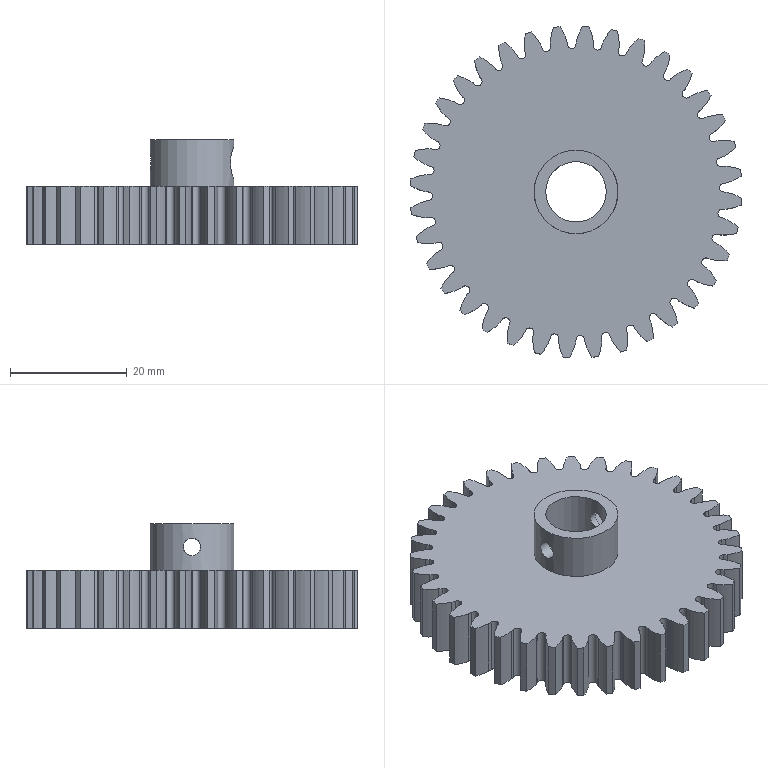Part | NX | features BREP 1, DATUM_CSYS 1 | 1 solid | 225 faces | box 56.956 x 56.956 x 18 mm | volume 22225 mm3 | cylinder 221 | plane 4 | commonest cylinder face diameters 6 x72 18.651 x72 1.45 x36 57 x36 3 x2 5.8 x1